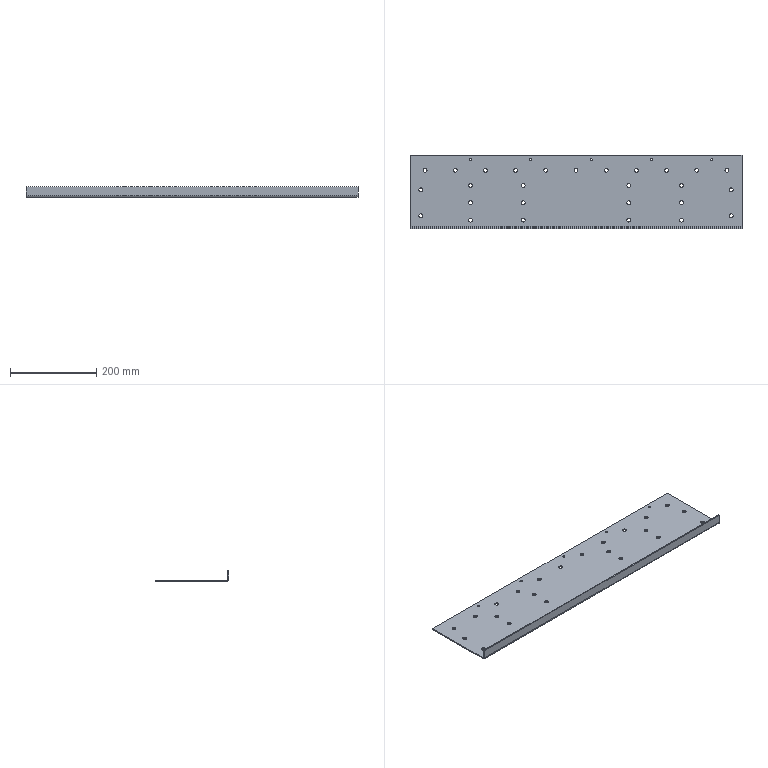Part | STEP file | cc-roller-10 | 1 solid | 42 faces | box 767.8 x 170 x 25 mm | volume 361884 mm3 | spline 32 | plane 8 | cylinder 2 | commonest cylinder face diameters 5 x1 10 x1